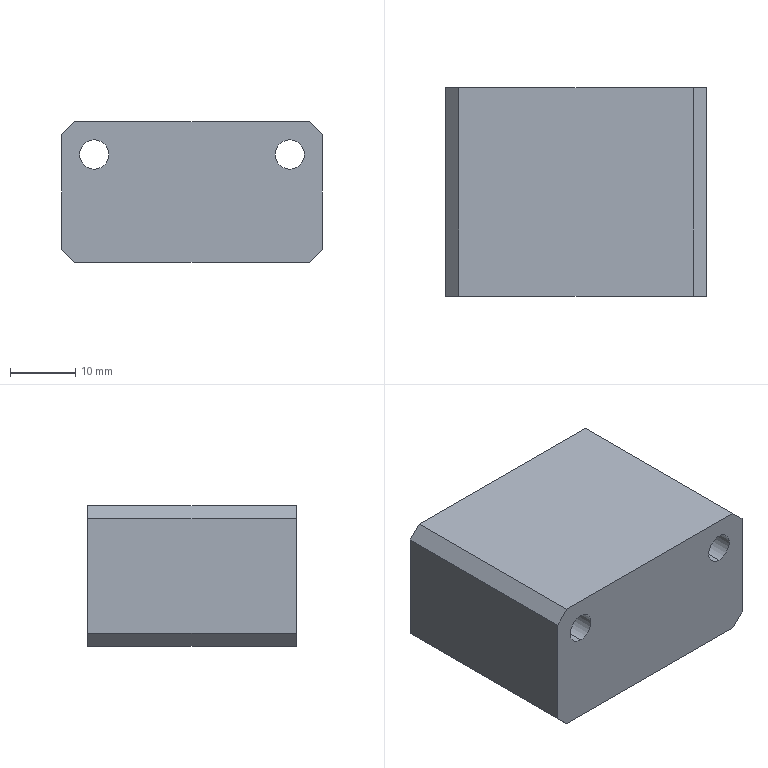Part | STEP file | PN_0036 | 1 solid | 28 faces | box 40 x 32 x 21.5 mm | volume 25854 mm3 | cylinder 12 | plane 12 | cone 4 | commonest cylinder face diameters 2.5 x4 4.5 x4 8 x4